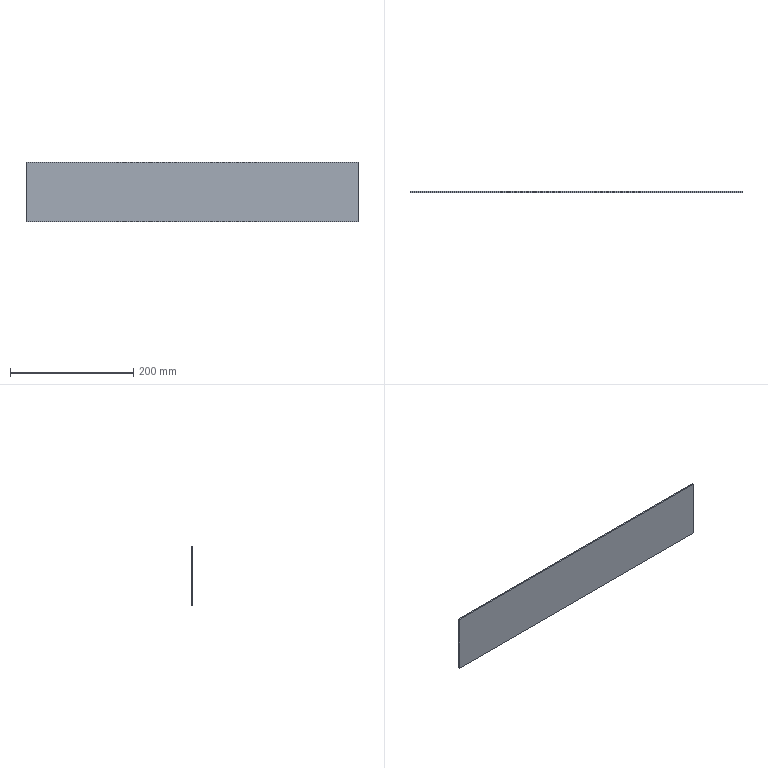Part | NX | 1 solid | 6 faces | box 538 x 2 x 97 mm | volume 104372 mm3 | plane 6
STEP:
#1=CARTESIAN_POINT('',(269.,0.,48.5));
#2=VERTEX_POINT('',#1);
#3=CARTESIAN_POINT('',(269.,0.,-48.5));
#4=VERTEX_POINT('',#3);
#5=CARTESIAN_POINT('',(269.,0.,-48.5));
#6=DIRECTION('',(0.,0.,-1.));
#7=VECTOR('',#6,1.);
#8=LINE('',#5,#7);
#9=EDGE_CURVE('',#2,#4,#8,.T.);
#10=ORIENTED_EDGE('',*,*,#9,.T.);
#11=CARTESIAN_POINT('',(269.,2.,-48.5));
#12=VERTEX_POINT('',#11);
#13=CARTESIAN_POINT('',(269.,2.,-48.5));
#14=DIRECTION('',(0.,-1.,0.));
#15=VECTOR('',#14,1.);
#16=LINE('',#13,#15);
#17=EDGE_CURVE('',#12,#4,#16,.T.);
#18=ORIENTED_EDGE('',*,*,#17,.F.);
#19=CARTESIAN_POINT('',(269.,2.,48.5));
#20=VERTEX_POINT('',#19);
#21=CARTESIAN_POINT('',(269.,2.,-48.5));
#22=DIRECTION('',(0.,0.,-1.));
#23=VECTOR('',#22,1.);
#24=LINE('',#21,#23);
#25=EDGE_CURVE('',#20,#12,#24,.T.);
#26=ORIENTED_EDGE('',*,*,#25,.F.);
#27=CARTESIAN_POINT('',(269.,2.,48.5));
#28=DIRECTION('',(0.,-1.,0.));
#29=VECTOR('',#28,1.);
#30=LINE('',#27,#29);
#31=EDGE_CURVE('',#20,#2,#30,.T.);
#32=ORIENTED_EDGE('',*,*,#31,.T.);
#33=EDGE_LOOP('',(#10,#18,#26,#32));
#34=FACE_OUTER_BOUND('',#33,.T.);
#35=CARTESIAN_POINT('',(269.,2.,-48.5));
#36=DIRECTION('',(-1.,0.,0.));
#37=DIRECTION('',(0.,0.,1.));
#38=AXIS2_PLACEMENT_3D('',#35,#36,#37);
#39=PLANE('',#38);
#40=ADVANCED_FACE('',(#34),#39,.F.);
#41=CARTESIAN_POINT('',(-269.,0.,-48.5));
#42=VERTEX_POINT('',#41);
#43=CARTESIAN_POINT('',(-269.,0.,-48.5));
#44=DIRECTION('',(-1.,0.,0.));
#45=VECTOR('',#44,1.);
#46=LINE('',#43,#45);
#47=EDGE_CURVE('',#4,#42,#46,.T.);
#48=ORIENTED_EDGE('',*,*,#47,.T.);
#49=CARTESIAN_POINT('',(-269.,2.,-48.5));
#50=VERTEX_POINT('',#49);
#51=CARTESIAN_POINT('',(-269.,2.,-48.5));
#52=DIRECTION('',(0.,-1.,0.));
#53=VECTOR('',#52,1.);
#54=LINE('',#51,#53);
#55=EDGE_CURVE('',#50,#42,#54,.T.);
#56=ORIENTED_EDGE('',*,*,#55,.F.);
#57=CARTESIAN_POINT('',(-269.,2.,-48.5));
#58=DIRECTION('',(-1.,0.,0.));
#59=VECTOR('',#58,1.);
#60=LINE('',#57,#59);
#61=EDGE_CURVE('',#12,#50,#60,.T.);
#62=ORIENTED_EDGE('',*,*,#61,.F.);
#63=ORIENTED_EDGE('',*,*,#17,.T.);
#64=EDGE_LOOP('',(#48,#56,#62,#63));
#65=FACE_OUTER_BOUND('',#64,.T.);
#66=CARTESIAN_POINT('',(-269.,2.,-48.5));
#67=DIRECTION('',(0.,0.,1.));
#68=DIRECTION('',(1.,0.,0.));
#69=AXIS2_PLACEMENT_3D('',#66,#67,#68);
#70=PLANE('',#69);
#71=ADVANCED_FACE('',(#65),#70,.F.);
#72=CARTESIAN_POINT('',(-269.,0.,48.5));
#73=VERTEX_POINT('',#72);
#74=CARTESIAN_POINT('',(-269.,0.,-48.5));
#75=DIRECTION('',(0.,0.,1.));
#76=VECTOR('',#75,1.);
#77=LINE('',#74,#76);
#78=EDGE_CURVE('',#42,#73,#77,.T.);
#79=ORIENTED_EDGE('',*,*,#78,.T.);
#80=CARTESIAN_POINT('',(-269.,2.,48.5));
#81=VERTEX_POINT('',#80);
#82=CARTESIAN_POINT('',(-269.,2.,48.5));
#83=DIRECTION('',(0.,-1.,0.));
#84=VECTOR('',#83,1.);
#85=LINE('',#82,#84);
#86=EDGE_CURVE('',#81,#73,#85,.T.);
#87=ORIENTED_EDGE('',*,*,#86,.F.);
#88=CARTESIAN_POINT('',(-269.,2.,-48.5));
#89=DIRECTION('',(0.,0.,1.));
#90=VECTOR('',#89,1.);
#91=LINE('',#88,#90);
#92=EDGE_CURVE('',#50,#81,#91,.T.);
#93=ORIENTED_EDGE('',*,*,#92,.F.);
#94=ORIENTED_EDGE('',*,*,#55,.T.);
#95=EDGE_LOOP('',(#79,#87,#93,#94));
#96=FACE_OUTER_BOUND('',#95,.T.);
#97=CARTESIAN_POINT('',(-269.,2.,-48.5));
#98=DIRECTION('',(1.,0.,0.));
#99=DIRECTION('',(0.,0.,-1.));
#100=AXIS2_PLACEMENT_3D('',#97,#98,#99);
#101=PLANE('',#100);
#102=ADVANCED_FACE('',(#96),#101,.F.);
#103=CARTESIAN_POINT('',(-269.,0.,48.5));
#104=DIRECTION('',(1.,0.,0.));
#105=VECTOR('',#104,1.);
#106=LINE('',#103,#105);
#107=EDGE_CURVE('',#73,#2,#106,.T.);
#108=ORIENTED_EDGE('',*,*,#107,.T.);
#109=ORIENTED_EDGE('',*,*,#31,.F.);
#110=CARTESIAN_POINT('',(-269.,2.,48.5));
#111=DIRECTION('',(1.,0.,0.));
#112=VECTOR('',#111,1.);
#113=LINE('',#110,#112);
#114=EDGE_CURVE('',#81,#20,#113,.T.);
#115=ORIENTED_EDGE('',*,*,#114,.F.);
#116=ORIENTED_EDGE('',*,*,#86,.T.);
#117=EDGE_LOOP('',(#108,#109,#115,#116));
#118=FACE_OUTER_BOUND('',#117,.T.);
#119=CARTESIAN_POINT('',(-269.,2.,48.5));
#120=DIRECTION('',(0.,0.,-1.));
#121=DIRECTION('',(-1.,0.,0.));
#122=AXIS2_PLACEMENT_3D('',#119,#120,#121);
#123=PLANE('',#122);
#124=ADVANCED_FACE('',(#118),#123,.F.);
#125=ORIENTED_EDGE('',*,*,#25,.T.);
#126=ORIENTED_EDGE('',*,*,#61,.T.);
#127=ORIENTED_EDGE('',*,*,#92,.T.);
#128=ORIENTED_EDGE('',*,*,#114,.T.);
#129=EDGE_LOOP('',(#125,#126,#127,#128));
#130=FACE_OUTER_BOUND('',#129,.T.);
#131=CARTESIAN_POINT('',(269.,2.,48.5));
#132=DIRECTION('',(0.,1.,0.));
#133=DIRECTION('',(0.,0.,1.));
#134=AXIS2_PLACEMENT_3D('',#131,#132,#133);
#135=PLANE('',#134);
#136=ADVANCED_FACE('',(#130),#135,.T.);
#137=ORIENTED_EDGE('',*,*,#9,.F.);
#138=ORIENTED_EDGE('',*,*,#107,.F.);
#139=ORIENTED_EDGE('',*,*,#78,.F.);
#140=ORIENTED_EDGE('',*,*,#47,.F.);
#141=EDGE_LOOP('',(#137,#138,#139,#140));
#142=FACE_OUTER_BOUND('',#141,.T.);
#143=CARTESIAN_POINT('',(269.,0.,48.5));
#144=DIRECTION('',(0.,1.,0.));
#145=DIRECTION('',(0.,0.,1.));
#146=AXIS2_PLACEMENT_3D('',#143,#144,#145);
#147=PLANE('',#146);
#148=ADVANCED_FACE('',(#142),#147,.F.);
#149=CLOSED_SHELL('',(#40,#71,#102,#124,#136,#148));
#150=MANIFOLD_SOLID_BREP('',#149);
#151=(LENGTH_UNIT()NAMED_UNIT(*)SI_UNIT(.MILLI.,.METRE.));
#152=UNCERTAINTY_MEASURE_WITH_UNIT(LENGTH_MEASURE(0.00002),#151,'','');
#153=(NAMED_UNIT(*)PLANE_ANGLE_UNIT()SI_UNIT($,.RADIAN.));
#154=PLANE_ANGLE_MEASURE_WITH_UNIT(PLANE_ANGLE_MEASURE(0.01745),#153);
#155=DIMENSIONAL_EXPONENTS(0.,0.,0.,0.,0.,0.,0.);
#156=(CONVERSION_BASED_UNIT('DEGREE',#154)NAMED_UNIT(#155)PLANE_ANGLE_UNIT());
#157=(NAMED_UNIT(*)SI_UNIT($,.STERADIAN.)SOLID_ANGLE_UNIT());
#158=(GEOMETRIC_REPRESENTATION_CONTEXT(3)GLOBAL_UNCERTAINTY_ASSIGNED_CONTEXT((#152))GLOBAL_UNIT_ASSIGNED_CONTEXT((#151,#156,#157))REPRESENTATION_CONTEXT('',''));
#159=ADVANCED_BREP_SHAPE_REPRESENTATION('',(#150),#158);